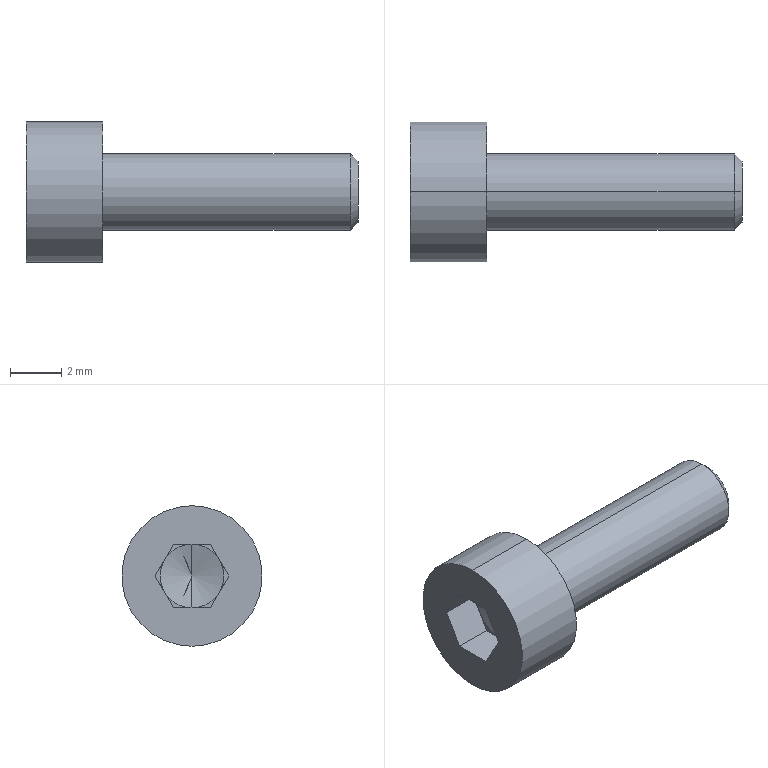Part | SolidWorks | features BaseBody 1 | 1 solid | 23 faces | box 13 x 5.5 x 5.5 mm | volume 132.881 mm3 | plane 15 | cylinder 4 | cone 4 | commonest cylinder face diameters 3 x2 5.5 x2
STEP:
#1=CARTESIAN_POINT('',(0.,0.,-1.5));
#2=VERTEX_POINT('',#1);
#3=CARTESIAN_POINT('',(0.,0.,1.5));
#4=VERTEX_POINT('',#3);
#5=CARTESIAN_POINT('',(0.,0.,0.));
#6=DIRECTION('',(1.,0.,0.));
#7=DIRECTION('',(0.,0.,-1.));
#8=AXIS2_PLACEMENT_3D('',#5,#6,#7);
#9=CIRCLE('',#8,1.5);
#10=EDGE_CURVE('',#2,#4,#9,.T.);
#11=ORIENTED_EDGE('',*,*,#10,.T.);
#12=CARTESIAN_POINT('',(9.694,0.,1.5));
#13=VERTEX_POINT('',#12);
#14=CARTESIAN_POINT('',(4.847,0.,1.5));
#15=DIRECTION('',(1.,0.,0.));
#16=VECTOR('',#15,1000.);
#17=LINE('',#14,#16);
#18=EDGE_CURVE('',#4,#13,#17,.T.);
#19=ORIENTED_EDGE('',*,*,#18,.T.);
#20=CARTESIAN_POINT('',(9.694,0.,-1.5));
#21=VERTEX_POINT('',#20);
#22=CARTESIAN_POINT('',(9.694,0.,0.));
#23=DIRECTION('',(-1.,0.,0.));
#24=DIRECTION('',(0.,0.,-1.));
#25=AXIS2_PLACEMENT_3D('',#22,#23,#24);
#26=CIRCLE('',#25,1.5);
#27=EDGE_CURVE('',#13,#21,#26,.T.);
#28=ORIENTED_EDGE('',*,*,#27,.T.);
#29=CARTESIAN_POINT('',(4.847,0.,-1.5));
#30=DIRECTION('',(1.,0.,0.));
#31=VECTOR('',#30,1000.);
#32=LINE('',#29,#31);
#33=EDGE_CURVE('',#2,#21,#32,.T.);
#34=ORIENTED_EDGE('',*,*,#33,.F.);
#35=EDGE_LOOP('',(#11,#19,#28,#34));
#36=FACE_OUTER_BOUND('',#35,.T.);
#37=CARTESIAN_POINT('',(4.847,0.,0.));
#38=DIRECTION('',(1.,0.,0.));
#39=DIRECTION('',(0.,0.,-1.));
#40=AXIS2_PLACEMENT_3D('',#37,#38,#39);
#41=CYLINDRICAL_SURFACE('',#40,1.5);
#42=ADVANCED_FACE('',(#36),#41,.T.);
#43=CARTESIAN_POINT('',(10.,0.,1.194));
#44=VERTEX_POINT('',#43);
#45=CARTESIAN_POINT('',(10.,0.,-1.194));
#46=VERTEX_POINT('',#45);
#47=CARTESIAN_POINT('',(10.,0.,0.));
#48=DIRECTION('',(-1.,0.,0.));
#49=DIRECTION('',(0.,0.,1.));
#50=AXIS2_PLACEMENT_3D('',#47,#48,#49);
#51=CIRCLE('',#50,1.194);
#52=EDGE_CURVE('',#44,#46,#51,.T.);
#53=ORIENTED_EDGE('',*,*,#52,.T.);
#54=CARTESIAN_POINT('',(9.694,0.,-1.5));
#55=DIRECTION('',(-0.7071,0.,-0.7071));
#56=VECTOR('',#55,1000.);
#57=LINE('',#54,#56);
#58=EDGE_CURVE('',#46,#21,#57,.T.);
#59=ORIENTED_EDGE('',*,*,#58,.T.);
#60=ORIENTED_EDGE('',*,*,#27,.F.);
#61=CARTESIAN_POINT('',(9.694,0.,1.5));
#62=DIRECTION('',(-0.7071,0.,0.7071));
#63=VECTOR('',#62,1000.);
#64=LINE('',#61,#63);
#65=EDGE_CURVE('',#44,#13,#64,.T.);
#66=ORIENTED_EDGE('',*,*,#65,.F.);
#67=EDGE_LOOP('',(#53,#59,#60,#66));
#68=FACE_OUTER_BOUND('',#67,.T.);
#69=CARTESIAN_POINT('',(9.694,0.,0.));
#70=DIRECTION('',(-1.,0.,0.));
#71=DIRECTION('',(0.,0.,1.));
#72=AXIS2_PLACEMENT_3D('',#69,#70,#71);
#73=CONICAL_SURFACE('',#72,1.5,0.7854);
#74=ADVANCED_FACE('',(#68),#73,.T.);
#75=CARTESIAN_POINT('',(-3.,0.,-2.75));
#76=VERTEX_POINT('',#75);
#77=CARTESIAN_POINT('',(-3.,0.,2.75));
#78=VERTEX_POINT('',#77);
#79=CARTESIAN_POINT('',(-3.,0.,0.));
#80=DIRECTION('',(1.,0.,0.));
#81=DIRECTION('',(0.,0.,-1.));
#82=AXIS2_PLACEMENT_3D('',#79,#80,#81);
#83=CIRCLE('',#82,2.75);
#84=EDGE_CURVE('',#76,#78,#83,.T.);
#85=ORIENTED_EDGE('',*,*,#84,.T.);
#86=CARTESIAN_POINT('',(0.,0.,2.75));
#87=VERTEX_POINT('',#86);
#88=CARTESIAN_POINT('',(-1.5,0.,2.75));
#89=DIRECTION('',(1.,0.,0.));
#90=VECTOR('',#89,1000.);
#91=LINE('',#88,#90);
#92=EDGE_CURVE('',#78,#87,#91,.T.);
#93=ORIENTED_EDGE('',*,*,#92,.T.);
#94=CARTESIAN_POINT('',(0.,0.,-2.75));
#95=VERTEX_POINT('',#94);
#96=CARTESIAN_POINT('',(0.,0.,0.));
#97=DIRECTION('',(1.,0.,0.));
#98=DIRECTION('',(0.,0.,-1.));
#99=AXIS2_PLACEMENT_3D('',#96,#97,#98);
#100=CIRCLE('',#99,2.75);
#101=EDGE_CURVE('',#95,#87,#100,.T.);
#102=ORIENTED_EDGE('',*,*,#101,.F.);
#103=CARTESIAN_POINT('',(-1.5,0.,-2.75));
#104=DIRECTION('',(1.,0.,0.));
#105=VECTOR('',#104,1000.);
#106=LINE('',#103,#105);
#107=EDGE_CURVE('',#76,#95,#106,.T.);
#108=ORIENTED_EDGE('',*,*,#107,.F.);
#109=EDGE_LOOP('',(#85,#93,#102,#108));
#110=FACE_OUTER_BOUND('',#109,.T.);
#111=CARTESIAN_POINT('',(-1.5,0.,0.));
#112=DIRECTION('',(1.,0.,0.));
#113=DIRECTION('',(0.,0.,-1.));
#114=AXIS2_PLACEMENT_3D('',#111,#112,#113);
#115=CYLINDRICAL_SURFACE('',#114,2.75);
#116=ADVANCED_FACE('',(#110),#115,.T.);
#117=CARTESIAN_POINT('',(-1.165,0.,0.));
#118=VERTEX_POINT('',#117);
#119=CARTESIAN_POINT('',(-1.5,0.,1.25));
#120=VERTEX_POINT('',#119);
#121=CARTESIAN_POINT('',(-1.5,0.,1.25));
#122=DIRECTION('',(-0.2588,0.,0.9659));
#123=VECTOR('',#122,1000.);
#124=LINE('',#121,#123);
#125=EDGE_CURVE('',#118,#120,#124,.T.);
#126=ORIENTED_EDGE('',*,*,#125,.F.);
#127=CARTESIAN_POINT('',(-1.5,0.,-1.25));
#128=VERTEX_POINT('',#127);
#129=CARTESIAN_POINT('',(-1.5,0.,-1.25));
#130=DIRECTION('',(-0.2588,0.,-0.9659));
#131=VECTOR('',#130,1000.);
#132=LINE('',#129,#131);
#133=EDGE_CURVE('',#118,#128,#132,.T.);
#134=ORIENTED_EDGE('',*,*,#133,.T.);
#135=CARTESIAN_POINT('',(-1.5,-1.083,-0.625));
#136=VERTEX_POINT('',#135);
#137=CARTESIAN_POINT('',(-1.5,0.,0.));
#138=DIRECTION('',(-1.,0.,0.));
#139=DIRECTION('',(0.,0.,1.));
#140=AXIS2_PLACEMENT_3D('',#137,#138,#139);
#141=CIRCLE('',#140,1.25);
#142=EDGE_CURVE('',#128,#136,#141,.T.);
#143=ORIENTED_EDGE('',*,*,#142,.T.);
#144=CARTESIAN_POINT('',(-1.5,-1.083,0.625));
#145=VERTEX_POINT('',#144);
#146=CARTESIAN_POINT('',(-1.5,0.,0.));
#147=DIRECTION('',(-1.,0.,0.));
#148=DIRECTION('',(0.,0.,1.));
#149=AXIS2_PLACEMENT_3D('',#146,#147,#148);
#150=CIRCLE('',#149,1.25);
#151=EDGE_CURVE('',#136,#145,#150,.T.);
#152=ORIENTED_EDGE('',*,*,#151,.T.);
#153=CARTESIAN_POINT('',(-1.5,0.,0.));
#154=DIRECTION('',(-1.,0.,0.));
#155=DIRECTION('',(0.,0.,1.));
#156=AXIS2_PLACEMENT_3D('',#153,#154,#155);
#157=CIRCLE('',#156,1.25);
#158=EDGE_CURVE('',#145,#120,#157,.T.);
#159=ORIENTED_EDGE('',*,*,#158,.T.);
#160=EDGE_LOOP('',(#126,#134,#143,#152,#159));
#161=FACE_OUTER_BOUND('',#160,.T.);
#162=CARTESIAN_POINT('',(-1.5,0.,0.));
#163=DIRECTION('',(-1.,0.,0.));
#164=DIRECTION('',(0.,0.,1.));
#165=AXIS2_PLACEMENT_3D('',#162,#163,#164);
#166=CONICAL_SURFACE('',#165,1.25,1.309);
#167=ADVANCED_FACE('',(#161),#166,.F.);
#168=ORIENTED_EDGE('',*,*,#18,.F.);
#169=CARTESIAN_POINT('',(0.,0.,0.));
#170=DIRECTION('',(1.,0.,0.));
#171=DIRECTION('',(0.,0.,-1.));
#172=AXIS2_PLACEMENT_3D('',#169,#170,#171);
#173=CIRCLE('',#172,1.5);
#174=EDGE_CURVE('',#4,#2,#173,.T.);
#175=ORIENTED_EDGE('',*,*,#174,.T.);
#176=ORIENTED_EDGE('',*,*,#33,.T.);
#177=CARTESIAN_POINT('',(9.694,0.,0.));
#178=DIRECTION('',(-1.,0.,0.));
#179=DIRECTION('',(0.,0.,-1.));
#180=AXIS2_PLACEMENT_3D('',#177,#178,#179);
#181=CIRCLE('',#180,1.5);
#182=EDGE_CURVE('',#21,#13,#181,.T.);
#183=ORIENTED_EDGE('',*,*,#182,.T.);
#184=EDGE_LOOP('',(#168,#175,#176,#183));
#185=FACE_OUTER_BOUND('',#184,.T.);
#186=CARTESIAN_POINT('',(4.847,0.,0.));
#187=DIRECTION('',(1.,0.,0.));
#188=DIRECTION('',(0.,0.,-1.));
#189=AXIS2_PLACEMENT_3D('',#186,#187,#188);
#190=CYLINDRICAL_SURFACE('',#189,1.5);
#191=ADVANCED_FACE('',(#185),#190,.T.);
#192=ORIENTED_EDGE('',*,*,#10,.F.);
#193=ORIENTED_EDGE('',*,*,#174,.F.);
#194=EDGE_LOOP('',(#192,#193));
#195=FACE_BOUND('',#194,.T.);
#196=ORIENTED_EDGE('',*,*,#101,.T.);
#197=CARTESIAN_POINT('',(0.,0.,0.));
#198=DIRECTION('',(1.,0.,0.));
#199=DIRECTION('',(0.,0.,-1.));
#200=AXIS2_PLACEMENT_3D('',#197,#198,#199);
#201=CIRCLE('',#200,2.75);
#202=EDGE_CURVE('',#87,#95,#201,.T.);
#203=ORIENTED_EDGE('',*,*,#202,.T.);
#204=EDGE_LOOP('',(#196,#203));
#205=FACE_OUTER_BOUND('',#204,.T.);
#206=CARTESIAN_POINT('',(0.,2.125,0.));
#207=DIRECTION('',(1.,0.,0.));
#208=DIRECTION('',(0.,0.,-1.));
#209=AXIS2_PLACEMENT_3D('',#206,#207,#208);
#210=PLANE('',#209);
#211=ADVANCED_FACE('',(#195,#205),#210,.T.);
#212=ORIENTED_EDGE('',*,*,#58,.F.);
#213=CARTESIAN_POINT('',(10.,0.,0.));
#214=DIRECTION('',(-1.,0.,0.));
#215=DIRECTION('',(0.,0.,1.));
#216=AXIS2_PLACEMENT_3D('',#213,#214,#215);
#217=CIRCLE('',#216,1.194);
#218=EDGE_CURVE('',#46,#44,#217,.T.);
#219=ORIENTED_EDGE('',*,*,#218,.T.);
#220=ORIENTED_EDGE('',*,*,#65,.T.);
#221=ORIENTED_EDGE('',*,*,#182,.F.);
#222=EDGE_LOOP('',(#212,#219,#220,#221));
#223=FACE_OUTER_BOUND('',#222,.T.);
#224=CARTESIAN_POINT('',(9.694,0.,0.));
#225=DIRECTION('',(-1.,0.,0.));
#226=DIRECTION('',(0.,0.,1.));
#227=AXIS2_PLACEMENT_3D('',#224,#225,#226);
#228=CONICAL_SURFACE('',#227,1.5,0.7854);
#229=ADVANCED_FACE('',(#223),#228,.T.);
#230=ORIENTED_EDGE('',*,*,#92,.F.);
#231=CARTESIAN_POINT('',(-3.,0.,0.));
#232=DIRECTION('',(1.,0.,0.));
#233=DIRECTION('',(0.,0.,-1.));
#234=AXIS2_PLACEMENT_3D('',#231,#232,#233);
#235=CIRCLE('',#234,2.75);
#236=EDGE_CURVE('',#78,#76,#235,.T.);
#237=ORIENTED_EDGE('',*,*,#236,.T.);
#238=ORIENTED_EDGE('',*,*,#107,.T.);
#239=ORIENTED_EDGE('',*,*,#202,.F.);
#240=EDGE_LOOP('',(#230,#237,#238,#239));
#241=FACE_OUTER_BOUND('',#240,.T.);
#242=CARTESIAN_POINT('',(-1.5,0.,0.));
#243=DIRECTION('',(1.,0.,0.));
#244=DIRECTION('',(0.,0.,-1.));
#245=AXIS2_PLACEMENT_3D('',#242,#243,#244);
#246=CYLINDRICAL_SURFACE('',#245,2.75);
#247=ADVANCED_FACE('',(#241),#246,.T.);
#248=ORIENTED_EDGE('',*,*,#52,.F.);
#249=ORIENTED_EDGE('',*,*,#218,.F.);
#250=EDGE_LOOP('',(#248,#249));
#251=FACE_OUTER_BOUND('',#250,.T.);
#252=CARTESIAN_POINT('',(10.,0.5968,0.));
#253=DIRECTION('',(1.,0.,0.));
#254=DIRECTION('',(0.,0.,-1.));
#255=AXIS2_PLACEMENT_3D('',#252,#253,#254);
#256=PLANE('',#255);
#257=ADVANCED_FACE('',(#251),#256,.T.);
#258=ORIENTED_EDGE('',*,*,#84,.F.);
#259=ORIENTED_EDGE('',*,*,#236,.F.);
#260=EDGE_LOOP('',(#258,#259));
#261=FACE_OUTER_BOUND('',#260,.T.);
#262=CARTESIAN_POINT('',(-3.,0.7217,-1.25));
#263=VERTEX_POINT('',#262);
#264=CARTESIAN_POINT('',(-3.,1.443,0.));
#265=VERTEX_POINT('',#264);
#266=CARTESIAN_POINT('',(-3.,0.7217,-1.25));
#267=DIRECTION('',(0.,0.5,0.866));
#268=VECTOR('',#267,1000.);
#269=LINE('',#266,#268);
#270=EDGE_CURVE('',#263,#265,#269,.T.);
#271=ORIENTED_EDGE('',*,*,#270,.T.);
#272=CARTESIAN_POINT('',(-3.,0.7217,1.25));
#273=VERTEX_POINT('',#272);
#274=CARTESIAN_POINT('',(-3.,1.443,0.));
#275=DIRECTION('',(0.,-0.5,0.866));
#276=VECTOR('',#275,1000.);
#277=LINE('',#274,#276);
#278=EDGE_CURVE('',#265,#273,#277,.T.);
#279=ORIENTED_EDGE('',*,*,#278,.T.);
#280=CARTESIAN_POINT('',(-3.,-0.7217,1.25));
#281=VERTEX_POINT('',#280);
#282=CARTESIAN_POINT('',(-3.,1.375,1.25));
#283=DIRECTION('',(0.,-1.,0.));
#284=VECTOR('',#283,1000.);
#285=LINE('',#282,#284);
#286=EDGE_CURVE('',#273,#281,#285,.T.);
#287=ORIENTED_EDGE('',*,*,#286,.T.);
#288=CARTESIAN_POINT('',(-3.,-1.443,0.));
#289=VERTEX_POINT('',#288);
#290=CARTESIAN_POINT('',(-3.,-0.7217,1.25));
#291=DIRECTION('',(0.,-0.5,-0.866));
#292=VECTOR('',#291,1000.);
#293=LINE('',#290,#292);
#294=EDGE_CURVE('',#281,#289,#293,.T.);
#295=ORIENTED_EDGE('',*,*,#294,.T.);
#296=CARTESIAN_POINT('',(-3.,-0.7217,-1.25));
#297=VERTEX_POINT('',#296);
#298=CARTESIAN_POINT('',(-3.,-1.443,0.));
#299=DIRECTION('',(0.,0.5,-0.866));
#300=VECTOR('',#299,1000.);
#301=LINE('',#298,#300);
#302=EDGE_CURVE('',#289,#297,#301,.T.);
#303=ORIENTED_EDGE('',*,*,#302,.T.);
#304=CARTESIAN_POINT('',(-3.,1.375,-1.25));
#305=DIRECTION('',(0.,1.,0.));
#306=VECTOR('',#305,1000.);
#307=LINE('',#304,#306);
#308=EDGE_CURVE('',#297,#263,#307,.T.);
#309=ORIENTED_EDGE('',*,*,#308,.T.);
#310=EDGE_LOOP('',(#271,#279,#287,#295,#303,#309));
#311=FACE_BOUND('',#310,.T.);
#312=CARTESIAN_POINT('',(-3.,1.375,0.));
#313=DIRECTION('',(-1.,0.,0.));
#314=DIRECTION('',(0.,0.,1.));
#315=AXIS2_PLACEMENT_3D('',#312,#313,#314);
#316=PLANE('',#315);
#317=ADVANCED_FACE('',(#261,#311),#316,.T.);
#318=CARTESIAN_POINT('',(-1.5,1.443,0.));
#319=VERTEX_POINT('',#318);
#320=CARTESIAN_POINT('',(-3.,1.443,0.));
#321=DIRECTION('',(-1.,0.,0.));
#322=VECTOR('',#321,1000.);
#323=LINE('',#320,#322);
#324=EDGE_CURVE('',#319,#265,#323,.T.);
#325=ORIENTED_EDGE('',*,*,#324,.F.);
#326=CARTESIAN_POINT('',(-1.5,1.083,0.625));
#327=VERTEX_POINT('',#326);
#328=CARTESIAN_POINT('',(-1.5,0.7217,1.25));
#329=DIRECTION('',(0.,0.5,-0.866));
#330=VECTOR('',#329,1000.);
#331=LINE('',#328,#330);
#332=EDGE_CURVE('',#327,#319,#331,.T.);
#333=ORIENTED_EDGE('',*,*,#332,.F.);
#334=CARTESIAN_POINT('',(-1.5,0.7217,1.25));
#335=VERTEX_POINT('',#334);
#336=CARTESIAN_POINT('',(-1.5,0.7217,1.25));
#337=DIRECTION('',(0.,0.5,-0.866));
#338=VECTOR('',#337,1000.);
#339=LINE('',#336,#338);
#340=EDGE_CURVE('',#335,#327,#339,.T.);
#341=ORIENTED_EDGE('',*,*,#340,.F.);
#342=CARTESIAN_POINT('',(-3.,0.7217,1.25));
#343=DIRECTION('',(1.,0.,0.));
#344=VECTOR('',#343,1000.);
#345=LINE('',#342,#344);
#346=EDGE_CURVE('',#273,#335,#345,.T.);
#347=ORIENTED_EDGE('',*,*,#346,.F.);
#348=ORIENTED_EDGE('',*,*,#278,.F.);
#349=EDGE_LOOP('',(#325,#333,#341,#347,#348));
#350=FACE_OUTER_BOUND('',#349,.T.);
#351=CARTESIAN_POINT('',(-3.,0.7217,1.25));
#352=DIRECTION('',(0.,0.866,0.5));
#353=DIRECTION('',(0.,-0.5,0.866));
#354=AXIS2_PLACEMENT_3D('',#351,#352,#353);
#355=PLANE('',#354);
#356=ADVANCED_FACE('',(#350),#355,.F.);
#357=CARTESIAN_POINT('',(-1.5,0.7217,-1.25));
#358=VERTEX_POINT('',#357);
#359=CARTESIAN_POINT('',(-3.,0.7217,-1.25));
#360=DIRECTION('',(-1.,0.,0.));
#361=VECTOR('',#360,1000.);
#362=LINE('',#359,#361);
#363=EDGE_CURVE('',#358,#263,#362,.T.);
#364=ORIENTED_EDGE('',*,*,#363,.F.);
#365=CARTESIAN_POINT('',(-1.5,1.083,-0.625));
#366=VERTEX_POINT('',#365);
#367=CARTESIAN_POINT('',(-1.5,1.443,0.));
#368=DIRECTION('',(0.,-0.5,-0.866));
#369=VECTOR('',#368,1000.);
#370=LINE('',#367,#369);
#371=EDGE_CURVE('',#366,#358,#370,.T.);
#372=ORIENTED_EDGE('',*,*,#371,.F.);
#373=CARTESIAN_POINT('',(-1.5,1.443,0.));
#374=DIRECTION('',(0.,-0.5,-0.866));
#375=VECTOR('',#374,1000.);
#376=LINE('',#373,#375);
#377=EDGE_CURVE('',#319,#366,#376,.T.);
#378=ORIENTED_EDGE('',*,*,#377,.F.);
#379=ORIENTED_EDGE('',*,*,#324,.T.);
#380=ORIENTED_EDGE('',*,*,#270,.F.);
#381=EDGE_LOOP('',(#364,#372,#378,#379,#380));
#382=FACE_OUTER_BOUND('',#381,.T.);
#383=CARTESIAN_POINT('',(-3.,1.443,0.));
#384=DIRECTION('',(0.,0.866,-0.5));
#385=DIRECTION('',(0.,0.5,0.866));
#386=AXIS2_PLACEMENT_3D('',#383,#384,#385);
#387=PLANE('',#386);
#388=ADVANCED_FACE('',(#382),#387,.F.);
#389=CARTESIAN_POINT('',(-1.5,-0.7217,-1.25));
#390=VERTEX_POINT('',#389);
#391=CARTESIAN_POINT('',(-3.,-0.7217,-1.25));
#392=DIRECTION('',(-1.,0.,0.));
#393=VECTOR('',#392,1000.);
#394=LINE('',#391,#393);
#395=EDGE_CURVE('',#390,#297,#394,.T.);
#396=ORIENTED_EDGE('',*,*,#395,.F.);
#397=CARTESIAN_POINT('',(-1.5,0.7217,-1.25));
#398=DIRECTION('',(0.,-1.,0.));
#399=VECTOR('',#398,1000.);
#400=LINE('',#397,#399);
#401=EDGE_CURVE('',#128,#390,#400,.T.);
#402=ORIENTED_EDGE('',*,*,#401,.F.);
#403=CARTESIAN_POINT('',(-1.5,0.7217,-1.25));
#404=DIRECTION('',(0.,-1.,0.));
#405=VECTOR('',#404,1000.);
#406=LINE('',#403,#405);
#407=EDGE_CURVE('',#358,#128,#406,.T.);
#408=ORIENTED_EDGE('',*,*,#407,.F.);
#409=ORIENTED_EDGE('',*,*,#363,.T.);
#410=ORIENTED_EDGE('',*,*,#308,.F.);
#411=EDGE_LOOP('',(#396,#402,#408,#409,#410));
#412=FACE_OUTER_BOUND('',#411,.T.);
#413=CARTESIAN_POINT('',(-3.,0.7217,-1.25));
#414=DIRECTION('',(0.,0.,-1.));
#415=DIRECTION('',(-1.,0.,0.));
#416=AXIS2_PLACEMENT_3D('',#413,#414,#415);
#417=PLANE('',#416);
#418=ADVANCED_FACE('',(#412),#417,.F.);
#419=CARTESIAN_POINT('',(-1.5,-1.443,0.));
#420=VERTEX_POINT('',#419);
#421=CARTESIAN_POINT('',(-3.,-1.443,0.));
#422=DIRECTION('',(-1.,0.,0.));
#423=VECTOR('',#422,1000.);
#424=LINE('',#421,#423);
#425=EDGE_CURVE('',#420,#289,#424,.T.);
#426=ORIENTED_EDGE('',*,*,#425,.F.);
#427=CARTESIAN_POINT('',(-1.5,-0.7217,-1.25));
#428=DIRECTION('',(0.,-0.5,0.866));
#429=VECTOR('',#428,1000.);
#430=LINE('',#427,#429);
#431=EDGE_CURVE('',#136,#420,#430,.T.);
#432=ORIENTED_EDGE('',*,*,#431,.F.);
#433=CARTESIAN_POINT('',(-1.5,-0.7217,-1.25));
#434=DIRECTION('',(0.,-0.5,0.866));
#435=VECTOR('',#434,1000.);
#436=LINE('',#433,#435);
#437=EDGE_CURVE('',#390,#136,#436,.T.);
#438=ORIENTED_EDGE('',*,*,#437,.F.);
#439=ORIENTED_EDGE('',*,*,#395,.T.);
#440=ORIENTED_EDGE('',*,*,#302,.F.);
#441=EDGE_LOOP('',(#426,#432,#438,#439,#440));
#442=FACE_OUTER_BOUND('',#441,.T.);
#443=CARTESIAN_POINT('',(-3.,-0.7217,-1.25));
#444=DIRECTION('',(0.,-0.866,-0.5));
#445=DIRECTION('',(0.,0.5,-0.866));
#446=AXIS2_PLACEMENT_3D('',#443,#444,#445);
#447=PLANE('',#446);
#448=ADVANCED_FACE('',(#442),#447,.F.);
#449=CARTESIAN_POINT('',(-1.5,-0.7217,1.25));
#450=VERTEX_POINT('',#449);
#451=CARTESIAN_POINT('',(-3.,-0.7217,1.25));
#452=DIRECTION('',(-1.,0.,0.));
#453=VECTOR('',#452,1000.);
#454=LINE('',#451,#453);
#455=EDGE_CURVE('',#450,#281,#454,.T.);
#456=ORIENTED_EDGE('',*,*,#455,.F.);
#457=CARTESIAN_POINT('',(-1.5,-1.443,0.));
#458=DIRECTION('',(0.,0.5,0.866));
#459=VECTOR('',#458,1000.);
#460=LINE('',#457,#459);
#461=EDGE_CURVE('',#145,#450,#460,.T.);
#462=ORIENTED_EDGE('',*,*,#461,.F.);
#463=CARTESIAN_POINT('',(-1.5,-1.443,0.));
#464=DIRECTION('',(0.,0.5,0.866));
#465=VECTOR('',#464,1000.);
#466=LINE('',#463,#465);
#467=EDGE_CURVE('',#420,#145,#466,.T.);
#468=ORIENTED_EDGE('',*,*,#467,.F.);
#469=ORIENTED_EDGE('',*,*,#425,.T.);
#470=ORIENTED_EDGE('',*,*,#294,.F.);
#471=EDGE_LOOP('',(#456,#462,#468,#469,#470));
#472=FACE_OUTER_BOUND('',#471,.T.);
#473=CARTESIAN_POINT('',(-3.,-1.443,0.));
#474=DIRECTION('',(0.,-0.866,0.5));
#475=DIRECTION('',(0.,-0.5,-0.866));
#476=AXIS2_PLACEMENT_3D('',#473,#474,#475);
#477=PLANE('',#476);
#478=ADVANCED_FACE('',(#472),#477,.F.);
#479=ORIENTED_EDGE('',*,*,#346,.T.);
#480=CARTESIAN_POINT('',(-1.5,-0.7217,1.25));
#481=DIRECTION('',(0.,1.,0.));
#482=VECTOR('',#481,1000.);
#483=LINE('',#480,#482);
#484=EDGE_CURVE('',#120,#335,#483,.T.);
#485=ORIENTED_EDGE('',*,*,#484,.F.);
#486=CARTESIAN_POINT('',(-1.5,-0.7217,1.25));
#487=DIRECTION('',(0.,1.,0.));
#488=VECTOR('',#487,1000.);
#489=LINE('',#486,#488);
#490=EDGE_CURVE('',#450,#120,#489,.T.);
#491=ORIENTED_EDGE('',*,*,#490,.F.);
#492=ORIENTED_EDGE('',*,*,#455,.T.);
#493=ORIENTED_EDGE('',*,*,#286,.F.);
#494=EDGE_LOOP('',(#479,#485,#491,#492,#493));
#495=FACE_OUTER_BOUND('',#494,.T.);
#496=CARTESIAN_POINT('',(-3.,-0.7217,1.25));
#497=DIRECTION('',(0.,0.,1.));
#498=DIRECTION('',(1.,0.,0.));
#499=AXIS2_PLACEMENT_3D('',#496,#497,#498);
#500=PLANE('',#499);
#501=ADVANCED_FACE('',(#495),#500,.F.);
#502=ORIENTED_EDGE('',*,*,#332,.T.);
#503=ORIENTED_EDGE('',*,*,#377,.T.);
#504=CARTESIAN_POINT('',(-1.5,0.,0.));
#505=DIRECTION('',(-1.,0.,0.));
#506=DIRECTION('',(0.,0.,1.));
#507=AXIS2_PLACEMENT_3D('',#504,#505,#506);
#508=CIRCLE('',#507,1.25);
#509=EDGE_CURVE('',#327,#366,#508,.T.);
#510=ORIENTED_EDGE('',*,*,#509,.F.);
#511=EDGE_LOOP('',(#502,#503,#510));
#512=FACE_OUTER_BOUND('',#511,.T.);
#513=CARTESIAN_POINT('',(-1.5,0.,0.));
#514=DIRECTION('',(1.,0.,0.));
#515=DIRECTION('',(0.,0.,-1.));
#516=AXIS2_PLACEMENT_3D('',#513,#514,#515);
#517=PLANE('',#516);
#518=ADVANCED_FACE('',(#512),#517,.F.);
#519=ORIENTED_EDGE('',*,*,#484,.T.);
#520=ORIENTED_EDGE('',*,*,#340,.T.);
#521=CARTESIAN_POINT('',(-1.5,0.,0.));
#522=DIRECTION('',(-1.,0.,0.));
#523=DIRECTION('',(0.,0.,1.));
#524=AXIS2_PLACEMENT_3D('',#521,#522,#523);
#525=CIRCLE('',#524,1.25);
#526=EDGE_CURVE('',#120,#327,#525,.T.);
#527=ORIENTED_EDGE('',*,*,#526,.F.);
#528=EDGE_LOOP('',(#519,#520,#527));
#529=FACE_OUTER_BOUND('',#528,.T.);
#530=CARTESIAN_POINT('',(-1.5,0.,0.));
#531=DIRECTION('',(1.,0.,0.));
#532=DIRECTION('',(0.,0.,-1.));
#533=AXIS2_PLACEMENT_3D('',#530,#531,#532);
#534=PLANE('',#533);
#535=ADVANCED_FACE('',(#529),#534,.F.);
#536=ORIENTED_EDGE('',*,*,#371,.T.);
#537=ORIENTED_EDGE('',*,*,#407,.T.);
#538=CARTESIAN_POINT('',(-1.5,0.,0.));
#539=DIRECTION('',(-1.,0.,0.));
#540=DIRECTION('',(0.,0.,1.));
#541=AXIS2_PLACEMENT_3D('',#538,#539,#540);
#542=CIRCLE('',#541,1.25);
#543=EDGE_CURVE('',#366,#128,#542,.T.);
#544=ORIENTED_EDGE('',*,*,#543,.F.);
#545=EDGE_LOOP('',(#536,#537,#544));
#546=FACE_OUTER_BOUND('',#545,.T.);
#547=CARTESIAN_POINT('',(-1.5,0.,0.));
#548=DIRECTION('',(1.,0.,0.));
#549=DIRECTION('',(0.,0.,-1.));
#550=AXIS2_PLACEMENT_3D('',#547,#548,#549);
#551=PLANE('',#550);
#552=ADVANCED_FACE('',(#546),#551,.F.);
#553=ORIENTED_EDGE('',*,*,#401,.T.);
#554=ORIENTED_EDGE('',*,*,#437,.T.);
#555=ORIENTED_EDGE('',*,*,#142,.F.);
#556=EDGE_LOOP('',(#553,#554,#555));
#557=FACE_OUTER_BOUND('',#556,.T.);
#558=CARTESIAN_POINT('',(-1.5,0.,0.));
#559=DIRECTION('',(1.,0.,0.));
#560=DIRECTION('',(0.,0.,-1.));
#561=AXIS2_PLACEMENT_3D('',#558,#559,#560);
#562=PLANE('',#561);
#563=ADVANCED_FACE('',(#557),#562,.F.);
#564=ORIENTED_EDGE('',*,*,#431,.T.);
#565=ORIENTED_EDGE('',*,*,#467,.T.);
#566=ORIENTED_EDGE('',*,*,#151,.F.);
#567=EDGE_LOOP('',(#564,#565,#566));
#568=FACE_OUTER_BOUND('',#567,.T.);
#569=CARTESIAN_POINT('',(-1.5,0.,0.));
#570=DIRECTION('',(1.,0.,0.));
#571=DIRECTION('',(0.,0.,-1.));
#572=AXIS2_PLACEMENT_3D('',#569,#570,#571);
#573=PLANE('',#572);
#574=ADVANCED_FACE('',(#568),#573,.F.);
#575=ORIENTED_EDGE('',*,*,#461,.T.);
#576=ORIENTED_EDGE('',*,*,#490,.T.);
#577=ORIENTED_EDGE('',*,*,#158,.F.);
#578=EDGE_LOOP('',(#575,#576,#577));
#579=FACE_OUTER_BOUND('',#578,.T.);
#580=CARTESIAN_POINT('',(-1.5,0.,0.));
#581=DIRECTION('',(1.,0.,0.));
#582=DIRECTION('',(0.,0.,-1.));
#583=AXIS2_PLACEMENT_3D('',#580,#581,#582);
#584=PLANE('',#583);
#585=ADVANCED_FACE('',(#579),#584,.F.);
#586=ORIENTED_EDGE('',*,*,#133,.F.);
#587=ORIENTED_EDGE('',*,*,#125,.T.);
#588=ORIENTED_EDGE('',*,*,#526,.T.);
#589=ORIENTED_EDGE('',*,*,#509,.T.);
#590=ORIENTED_EDGE('',*,*,#543,.T.);
#591=EDGE_LOOP('',(#586,#587,#588,#589,#590));
#592=FACE_OUTER_BOUND('',#591,.T.);
#593=CARTESIAN_POINT('',(-1.5,0.,0.));
#594=DIRECTION('',(-1.,0.,0.));
#595=DIRECTION('',(0.,0.,1.));
#596=AXIS2_PLACEMENT_3D('',#593,#594,#595);
#597=CONICAL_SURFACE('',#596,1.25,1.309);
#598=ADVANCED_FACE('',(#592),#597,.F.);
#599=CLOSED_SHELL('',(#42,#74,#116,#167,#191,#211,#229,#247,#257,#317,#356,#388,#418,#448,#478,#501,#518,#535,#552,#563,#574,#585,#598));
#600=MANIFOLD_SOLID_BREP('',#599);
#601=CARTESIAN_POINT('',(0.,0.,0.));
#602=DIRECTION('',(0.,0.,1.));
#603=DIRECTION('',(1.,0.,0.));
#604=AXIS2_PLACEMENT_3D('',#601,#602,#603);
#605=(LENGTH_UNIT()NAMED_UNIT(*)SI_UNIT(.MILLI.,.METRE.));
#606=UNCERTAINTY_MEASURE_WITH_UNIT(LENGTH_MEASURE(0.00001),#605,'','');
#607=(NAMED_UNIT(*)PLANE_ANGLE_UNIT()SI_UNIT($,.RADIAN.));
#608=(NAMED_UNIT(*)SI_UNIT($,.STERADIAN.)SOLID_ANGLE_UNIT());
#609=(GEOMETRIC_REPRESENTATION_CONTEXT(3)GLOBAL_UNCERTAINTY_ASSIGNED_CONTEXT((#606))GLOBAL_UNIT_ASSIGNED_CONTEXT((#605,#607,#608))REPRESENTATION_CONTEXT('',''));
#610=ADVANCED_BREP_SHAPE_REPRESENTATION('',(#600,#604),#609);